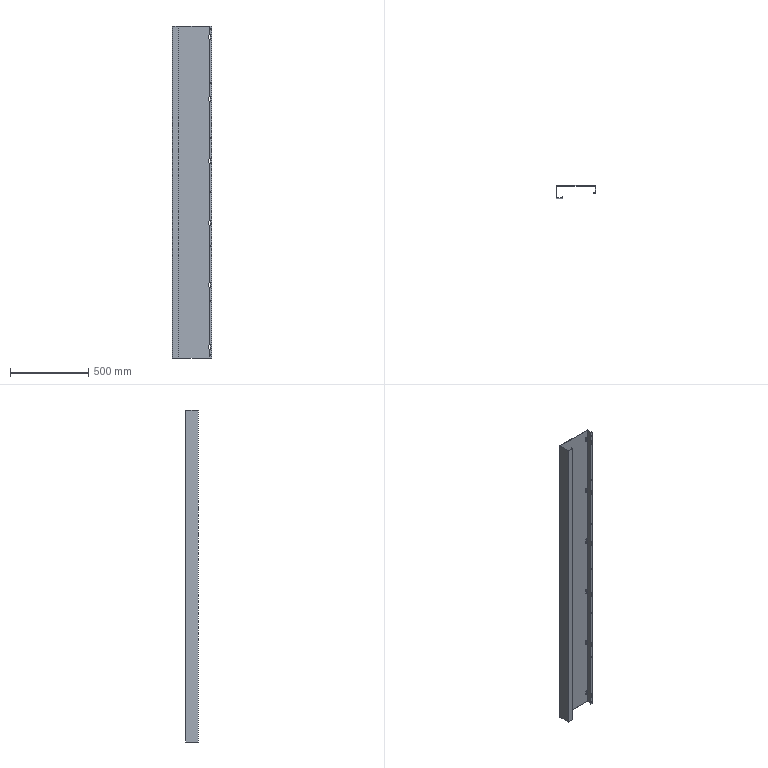Part | SolidWorks | features ICE 5, Cut 3, EdgeFlange 2, Fillet 1, FlatPattern 1, MirrorPattern 1, SMBaseFlange 1, SheetMetal 1 | 1 solid | 128 faces | box 250 x 80 x 2116 mm | volume 1092548 mm3 | plane 72 | cylinder 56 | commonest cylinder face diameters 6.2 x28 9 x18 1 x5 3.4 x5